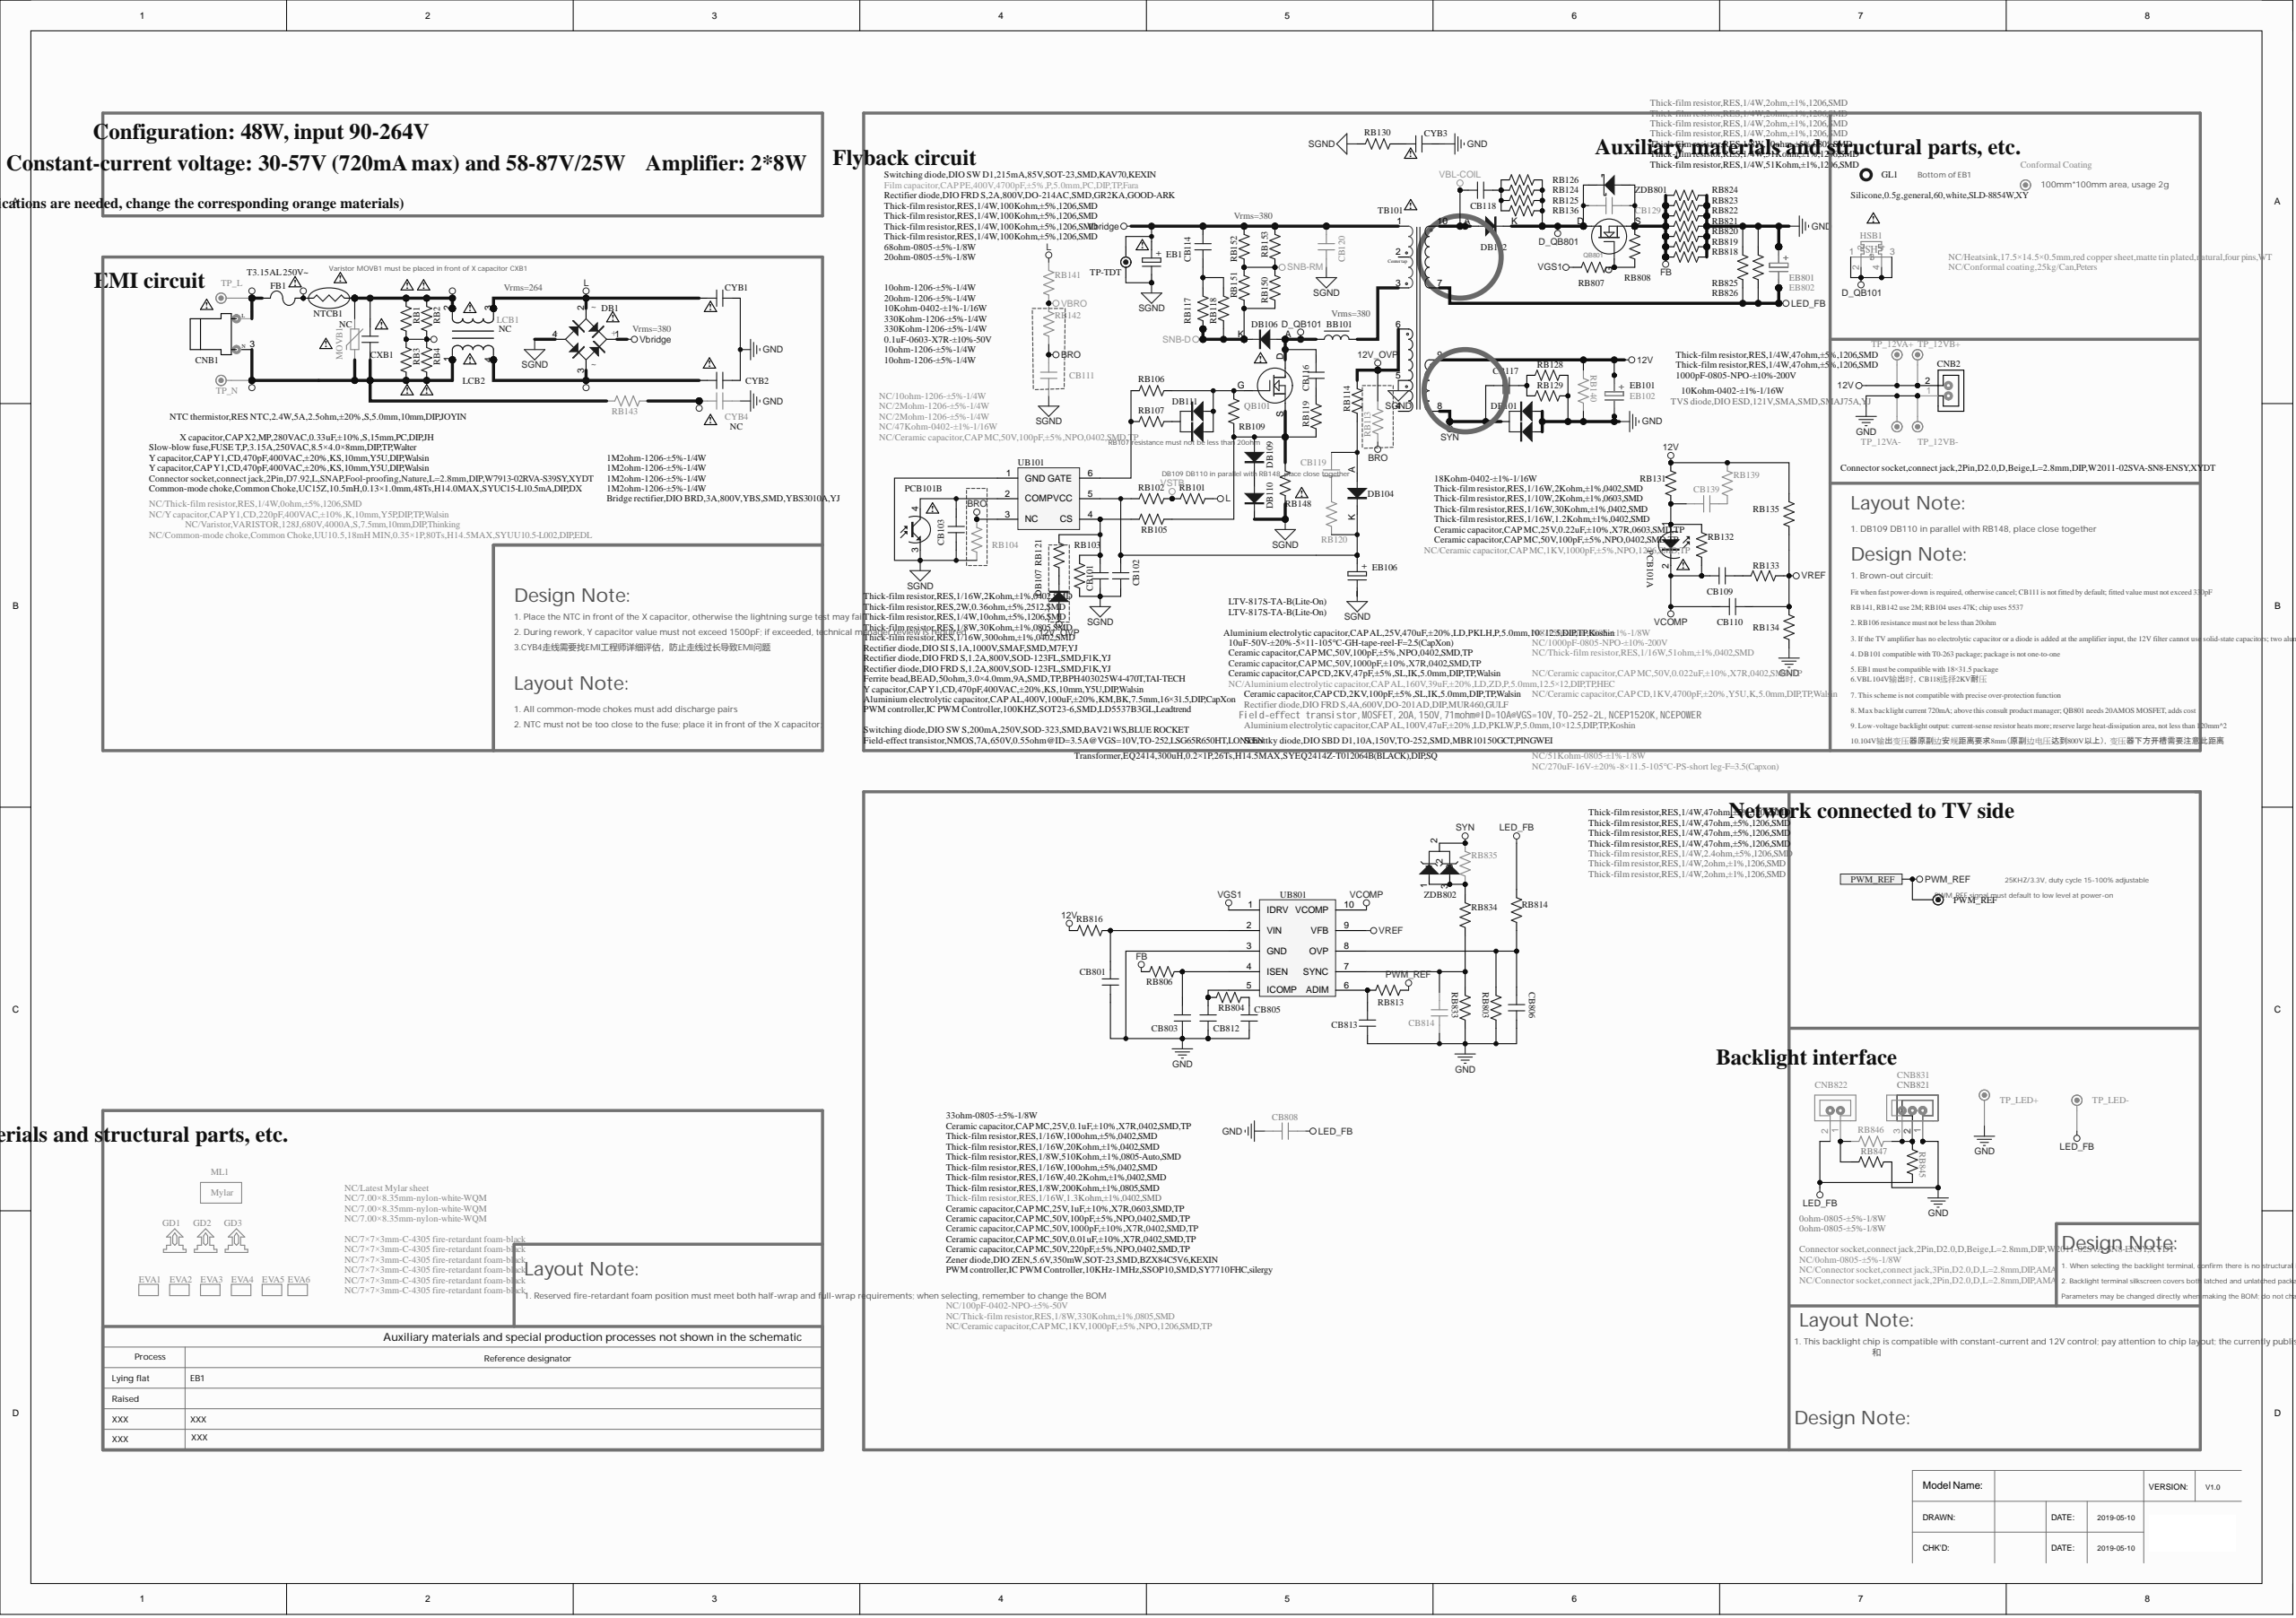Circuit board | Altium Designer | 578 parts | 300 nets | one sheet of the schematic
Parts on this sheet (reference | value | footprint):
BB101 | Ferrite bead,BEAD,50ohm,3.0×4.0mm,9A,SMD,TP,BPH403025W4-470T,TAI-TECH | L(4*3*2.55)-S
CB101 | Ceramic capacitor,CAP MC,50V,100pF,±5%,NPO,0402,SMD,TP | C0402
CB102 | 0.1uF-0603-X7R-±10%-50V | C0603
CB103 | Ceramic capacitor,CAP MC,50V,1000pF,±10%,X7R,0402,SMD,TP | C0402
CB109 | Ceramic capacitor,CAP MC,25V,0.22uF,±10%,X7R,0603,SMD,TP | C0603
CB110 | Ceramic capacitor,CAP MC,50V,100pF,±5%,NPO,0402,SMD,TP | C0402
CB111 | NC/Ceramic capacitor,CAP MC,50V,100pF,±5%,NPO,0402,SMD,TP | C0402
CB114 | Film capacitor,CAP PE,400V,4700pF,±5%,P,5.0mm,PC,DIP,TP,Fara | CAP8*2.5-V-5
CB116 | Ceramic capacitor,CAP CD,2KV,47pF,±5%,SL,IK,5.0mm,DIP,TP,Walsin | CAP7.5*5-V-5-1
CB117 | 1000pF-0805-NPO-±10%-200V | C0805
CB118 | Ceramic capacitor,CAP CD,2KV,100pF,±5%,SL,IK,5.0mm,DIP,TP,Walsin | CAP8.5*5-V-5
CB119 | NC/1000pF-0805-NPO-±10%-200V | C0805
CB120 | NC/Ceramic capacitor,CAP CD,1KV,4700pF,±20%,Y5U,K,5.0mm,DIP,TP,Walsin | CAP10*4.5-V-5
CB129 | NC/Ceramic capacitor,CAP MC,1KV,1000pF,±5%,NPO,1206,SMD,TP | C1206
CB139 | NC/Ceramic capacitor,CAP MC,50V,0.022uF,±10%,X7R,0402,SMD,TP | C0603
CB801 | Ceramic capacitor,CAP MC,25V,1uF,±10%,X7R,0603,SMD,TP | C0603
CB803 | Ceramic capacitor,CAP MC,25V,0.1uF,±10%,X7R,0402,SMD,TP | C0402
CB805 | Ceramic capacitor,CAP MC,50V,0.01uF,±10%,X7R,0402,SMD,TP | C0402
CB806 | Ceramic capacitor,CAP MC,50V,1000pF,±10%,X7R,0402,SMD,TP | C0402
CB808 | NC/Ceramic capacitor,CAP MC,1KV,1000pF,±5%,NPO,1206,SMD,TP | C1206
CB812 | Ceramic capacitor,CAP MC,50V,220pF,±5%,NPO,0402,SMD,TP | C0402
CB813 | Ceramic capacitor,CAP MC,50V,100pF,±5%,NPO,0402,SMD,TP | C0402
CB814 | NC/100pF-0402-NPO-±5%-50V | C0402
CNB1 | Connector socket,connect jack,2Pin,D7.92,L,SNAP,Fool-proofing,Nature,L=2.8mm,DIP,W7913-02RVA-S39SY,XYDT | CON2-H7.92
CNB2 | Connector socket,connect jack,2Pin,D2.0,D,Beige,L=2.8mm,DIP,W2011-02SVA-SN8-ENSY,XYDT | SIP2/2.0D-1
CNB821 | Connector socket,connect jack,2Pin,D2.0,D,Beige,L=2.8mm,DIP,W2011-02SVA-SN8-ENSY,XYDT | SIP2/2.0D-CP
CNB822 | NC/Connector socket,connect jack,2Pin,D2.0,D,L=2.8mm,DIP,AMA | SIP2/2.0D-CP
CNB831 | NC/Connector socket,connect jack,3Pin,D2.0,D,L=2.8mm,DIP,AMA | SIP3/2.0D-CP
CXB1 | X capacitor,CAP X2,MP,280VAC,0.33uF,±10%,S,15mm,PC,DIP,JH | CAP18*8.5-V-15
CYB1 | Y capacitor,CAP Y1,CD,470pF,400VAC,±20%,KS,10mm,Y5U,DIP,Walsin | CAP13*5-V-10-1
CYB2 | Y capacitor,CAP Y1,CD,470pF,400VAC,±20%,KS,10mm,Y5U,DIP,Walsin | CAP13*5-V-10-1
CYB3 | Y capacitor,CAP Y1,CD,470pF,400VAC,±20%,KS,10mm,Y5U,DIP,Walsin | CAP13*5-V-10-1
CYB4 | NC/Y capacitor,CAP Y1,CD,220pF,400VAC,±10%,K,10mm,Y5P,DIP,TP,Walsin | CAP13*5-V-10-1
DB1 | Bridge rectifier,DIO BRD,3A,800V,YBS,SMD,YBS3010A,YJ | B/YBS3010A
DB101 | Schottky diode,DIO SBD D1,10A,150V,TO-252,SMD,MBR10150GCT,PINGWEI | D2PAK3
DB102 | Rectifier diode,DIO FRD S,4A,600V,DO-201AD,DIP,MUR460,GULF | D3-H-20
DB104 | Rectifier diode,DIO SI S,1A,1000V,SMAF,SMD,M7F,YJ | DIODE-S-2
DB106 | Rectifier diode,DIO FRD S,2A,800V,DO-214AC,SMD,GR2KA,GOOD-ARK | DIODE-SMA-2
DB107 | Switching diode,DIO SW S,200mA,250V,SOD-323,SMD,BAV21WS,BLUE ROCKET | DIODE-S-12
DB109 | Rectifier diode,DIO FRD S,1.2A,800V,SOD-123FL,SMD,F1K,YJ | DIODE-S-14
DB110 | Rectifier diode,DIO FRD S,1.2A,800V,SOD-123FL,SMD,F1K,YJ | DIODE-S-14
DB111 | Switching diode,DIO SW D1,215mA,85V,SOT-23,SMD,KAV70,KEXIN | SO-23
EB1 | Aluminium electrolytic capacitor,CAP AL,400V,100uF,±20%,KM,BK,7.5mm,16×31.5,DIP,CapXon | EC(18*31.5)-H-7.5
EB101 | Aluminium electrolytic capacitor,CAP AL,25V,470uF,±20%,LD,PKLH,P,5.0mm,10×12.5,DIP,TP,Koshin | EC(10*12.5)-V-5
EB102 | NC/270uF-16V-±20%-8×11.5-105℃-PS-short leg-F=3.5(Capxon) | EC(8*11)-V-3.5
EB106 | 10uF-50V-±20%-5×11-105℃-GH-tape-reel-F=2.5(CapXon) | EC(5*11)-V-2.5
EB801 | Aluminium electrolytic capacitor,CAP AL,100V,47uF,±20%,LD,PKLW,P,5.0mm,10×12.5,DIP,TP,Koshin | EC(10*12.5)-V-5
EB802 | NC/Aluminium electrolytic capacitor,CAP AL,160V,39uF,±20%,LD,ZD,P,5.0mm,12.5×12,DIP,TP,HEC | EC(13*13)-V-5
EVA1 | NC/7×7×3mm-C-4305 fire-retardant foam-black | EVA(7*7*3)
EVA2 | NC/7×7×3mm-C-4305 fire-retardant foam-black | EVA(7*7*3)
EVA3 | NC/7×7×3mm-C-4305 fire-retardant foam-black | EVA(7*7*3)
EVA4 | NC/7×7×3mm-C-4305 fire-retardant foam-black | EVA(7*7*3)
EVA5 | NC/7×7×3mm-C-4305 fire-retardant foam-black | EVA(7*7*3)
EVA6 | NC/7×7×3mm-C-4305 fire-retardant foam-black | EVA(7*7*3)
FB1 | Slow-blow fuse,FUSE T,P,3.15A,250VAC,8.5×4.0×8mm,DIP,TP,Walter | FUSE8.5*4-V-5(T3.15AL 250V~)
GD1 | NC/7.00×8.35mm-nylon-white-WQM | Fixed
GD2 | NC/7.00×8.35mm-nylon-white-WQM | Fixed
GD3 | NC/7.00×8.35mm-nylon-white-WQM | Fixed
GL1 | Silicone,0.5g,general,60,white,SLD-8854W,XY | Silica gel-15
HSB1 | NC/Heatsink,17.5×14.5×0.5mm,red copper sheet,matte tin plated,natural,four pins,WT | HS149-YZ
LCB1 | NC/Common-mode choke,Common Choke,UU10.5,18mH MIN,0.35×1P,80Ts,H14.5MAX,SYUU10.5-L002,DIP,EDL | L/UU10.5/10*13-2
LCB2 | Common-mode choke,Common Choke,UC15Z,10.5mH,0.13×1.0mm,48Ts,H14.0MAX,SYUC15-L10.5mA,DIP,DX | L/LC4/20.5*16-H-17*9(12.9)
ML1 | NC/Latest Mylar sheet | Mylar
MOVB1 | NC/Varistor,VARISTOR,128J,680V,4000A,S,7.5mm,10mm,DIP,Thinking | VR(13*5)-V-7.5
NTCB1 | NTC thermistor,RES NTC,2.4W,5A,2.5ohm,±20%,S,5.0mm,10mm,DIP,JOYIN | NTC(10*5)-V5
QB101 | Field-effect transistor,NMOS,7A,650V,0.55ohm@ID=3.5A@VGS=10V,TO-252,LSG65R650HT,LONTEN | TO-252-GDS
QB801 | Field-effect transistor,MOSFET,20A,150V,71mohm@ID=10A@VGS=10V,TO-252-2L,NCEP1520K,NCEPOWER | TO-252-GDS
RB1 | 1M2ohm-1206-±5%-1/4W | R1206
RB2 | 1M2ohm-1206-±5%-1/4W | R1206
RB3 | 1M2ohm-1206-±5%-1/4W | R1206
RB4 | 1M2ohm-1206-±5%-1/4W | R1206
RB101 | 330Kohm-1206-±5%-1/4W | R1206
RB102 | 330Kohm-1206-±5%-1/4W | R1206
RB103 | Thick-film resistor,RES,1/16W,2Kohm,±1%,0402,SMD | R0402
RB104 | NC/47Kohm-0402-±1%-1/16W | R0402
RB105 | Thick-film resistor,RES,1/16W,300ohm,±1%,0402,SMD | R0402
RB106 | 68ohm-0805-±5%-1/8W | R0805
RB107 | 20ohm-0805-±5%-1/8W | R0805
RB109 | 10Kohm-0402-±1%-1/16W | R0402
RB113 | NC/150Kohm-0805-±1%-1/8W | R0805
RB114 | Thick-film resistor,RES,1/4W,10ohm,±5%,1206,SMD | R1206
RB117 | 10ohm-1206-±5%-1/4W | R1206
RB118 | 10ohm-1206-±5%-1/4W | R1206
RB119 | 10ohm-1206-±5%-1/4W | R1206
RB120 | NC/10ohm-1206-±5%-1/4W | R1206
RB121 | Thick-film resistor,RES,1/8W,30Kohm,±1%,0805,SMD | R0805
RB124 | Thick-film resistor,RES,1/4W,47ohm,±5%,1206,SMD | R1206
RB125 | Thick-film resistor,RES,1/4W,47ohm,±5%,1206,SMD | R1206
RB126 | Thick-film resistor,RES,1/4W,47ohm,±5%,1206,SMD | R1206
RB128 | Thick-film resistor,RES,1/4W,47ohm,±5%,1206,SMD | R1206
RB129 | Thick-film resistor,RES,1/4W,47ohm,±5%,1206,SMD | R1206
RB130 | 20ohm-1206-±5%-1/4W | R1206
RB131 | Thick-film resistor,RES,1/10W,2Kohm,±1%,0603,SMD | R0603
RB132 | Thick-film resistor,RES,1/16W,1.2Kohm,±1%,0402,SMD | R0402
RB133 | Thick-film resistor,RES,1/16W,30Kohm,±1%,0402,SMD | R0402
RB134 | Thick-film resistor,RES,1/16W,2Kohm,±1%,0402,SMD | R0402
RB135 | 18Kohm-0402-±1%-1/16W | R0402
RB136 | Thick-film resistor,RES,1/4W,47ohm,±5%,1206,SMD | R1206
RB139 | NC/Thick-film resistor,RES,1/16W,51ohm,±1%,0402,SMD | R0402
RB140 | NC/51Kohm-0805-±1%-1/8W | R0805
RB141 | NC/2Mohm-1206-±5%-1/4W | R1206
RB142 | NC/2Mohm-1206-±5%-1/4W | R1206
RB143 | NC/Thick-film resistor,RES,1/4W,0ohm,±5%,1206,SMD | R1206
RB148 | Thick-film resistor,RES,2W,0.36ohm,±5%,2512,SMD | R2512-1
RB150 | Thick-film resistor,RES,1/4W,100Kohm,±5%,1206,SMD | R1206
RB151 | Thick-film resistor,RES,1/4W,100Kohm,±5%,1206,SMD | R1206
RB152 | Thick-film resistor,RES,1/4W,100Kohm,±5%,1206,SMD | R1206
RB153 | Thick-film resistor,RES,1/4W,100Kohm,±5%,1206,SMD | R1206
RB803 | Thick-film resistor,RES,1/16W,1.3Kohm,±1%,0402,SMD | R0402
RB804 | Thick-film resistor,RES,1/16W,20Kohm,±1%,0402,SMD | R0402
RB806 | Thick-film resistor,RES,1/16W,100ohm,±5%,0402,SMD | R0402
RB807 | Thick-film resistor,RES,1/8W,10ohm,±5%,0805,SMD | R0805
RB808 | 10Kohm-0402-±1%-1/16W | R0402
RB813 | Thick-film resistor,RES,1/16W,100ohm,±5%,0402,SMD | R0402
RB814 | Thick-film resistor,RES,1/8W,510Kohm,±1%,0805-Auto,SMD | R0805
RB816 | 33ohm-0805-±5%-1/8W | R0805
RB818 | Thick-film resistor,RES,1/4W,2ohm,±1%,1206,SMD | R1206
RB819 | Thick-film resistor,RES,1/4W,2ohm,±1%,1206,SMD | R1206
RB820 | Thick-film resistor,RES,1/4W,2ohm,±1%,1206,SMD | R1206
RB821 | Thick-film resistor,RES,1/4W,2ohm,±1%,1206,SMD | R1206
RB822 | Thick-film resistor,RES,1/4W,2ohm,±1%,1206,SMD | R1206
RB823 | Thick-film resistor,RES,1/4W,2ohm,±1%,1206,SMD | R1206
RB824 | Thick-film resistor,RES,1/4W,2.4ohm,±5%,1206,SMD | R1206
RB825 | Thick-film resistor,RES,1/4W,51Kohm,±1%,1206,SMD | R1206
RB826 | Thick-film resistor,RES,1/4W,51Kohm,±1%,1206,SMD | R1206
RB833 | Thick-film resistor,RES,1/16W,40.2Kohm,±1%,0402,SMD | R0402
RB834 | Thick-film resistor,RES,1/8W,200Kohm,±1%,0805,SMD | R0805
RB835 | NC/Thick-film resistor,RES,1/8W,330Kohm,±1%,0805,SMD | R0805
RB845 | 0ohm-0805-±5%-1/8W | R0805
RB846 | NC/0ohm-0805-±5%-1/8W | R0805
RB847 | 0ohm-0805-±5%-1/8W | R0805
TB101 | Transformer,EQ2414,300uH,0.2×1P,26Ts,H14.5MAX,SYEQ2414Z-T012064B(BLACK),DIP,SQ | T/EQ2414*10
TP-TDT | TP-TDT
TP_12VA+ | NC/ | TP
TP_12VA- | NC/ | TP
TP_L | NC/ | TP-80
TP_LED+ | NC/ | TP
TP_N | NC/ | TP-80
UB101 | PWM controller,IC PWM Controller,100KHZ,SOT23-6,SMD,LD5537B3GL,Leadtrend | SOT-26
UB801 | PWM controller,IC PWM Controller,10KHz-1MHz,SSOP10,SMD,SY7710FHC,silergy | SOP10/1.0-1
ZDB801 | TVS diode,DIO ESD,121V,SMA,SMD,SMAJ75A,YJ | DIODE-SMA-1
ZDB802 | Zener diode,DIO ZEN,5.6V,350mW,SOT-23,SMD,BZX84C5V6,KEXIN | SO-23
Nets of these parts (net: part-pin ...):
VSTB: RB101-2 RB102-2
VREF: CB110-2 RB133-1 RB134-2 RB135-2 UB801-9
VGS1: RB807-1 UB801-1
VCOMP: CB109-1 CB110-1 RB132-1 UB801-10
VBRO: RB141-1 RB142-2
Vbridge: CB114-1 CB120-2 DB1-1 EB1-1 RB152-2 RB153-2 TB101-1 TP-TDT-1
VBL-COIL: CB118-1 DB102-A TB101-10
SYN: CB117-1 DB101-2 RB835-1 TB101-8 ZDB802-2
SNB-RM: RB150-2 RB151-2 RB152-1 RB153-1
SNB-D: DB106-K RB117-1 RB118-1 RB150-1 RB151-1
SGND: CB101-2 CB102-2 CB103-2 CB111-1 CB120-1 DB1-4 DB110-K EB1-2 EB106-2 RB103-1 RB104-1 RB130-1 RB148-1 TB101-5 TP-TDT-2 UB101-1
PWM_REF: RB813-1
NetRB834_2: RB834-2 RB835-2 ZDB802-1 ZDB802-3
NetRB106_1: RB106-1 RB107-1 UB101-6
NetQB801_G: QB801-G RB807-2 RB808-1
NetDB111_2: DB111-2 RB107-2
NetDB111_1: DB111-1 DB111-3 QB101-G RB106-2 RB109-2
NetDB109_K: DB109-K DB110-A
NetDB109_A: DB109-A QB101-S RB105-2 RB109-1 RB119-1 RB148-2
NetDB107_K: DB107-K RB121-1
NetCYB3_1: CYB3-1 RB130-2
NetCNB822_1: CNB822-1 RB846-2 RB847-2
NetCNB821_2: CNB821-2 CNB831-2 CNB831-3 RB845-2 RB846-1
NetCB814_1: CB814-1 RB833-2 RB834-1 UB801-7
NetCB813_2: CB813-2 RB813-2 UB801-6
NetCB812_2: CB812-2 RB804-2 UB801-5
NetCB806_1: CB806-1 RB803-2 RB814-2 UB801-8
NetCB805_2: CB805-2 RB804-1
NetCB803_1: CB803-1 RB806-2 UB801-4
NetCB801_1: CB801-1 RB816-2 UB801-2
NetCB139_2: CB139-2 RB131-1 RB132-2
NetCB139_1: CB139-1 RB139-2
NetCB119_2: CB119-2 DB104-A RB114-1
NetCB119_1: CB119-1 RB120-2
NetCB118_2: CB118-2 RB124-2 RB125-2 RB126-2 RB136-2
NetCB117_2: CB117-2 RB128-1 RB129-1
NetCB116_2: CB116-2 RB119-2
NetCB114_2: CB114-2 RB117-2 RB118-2
NetCB109_2: CB109-2 RB133-2
NetCB103_1: CB103-1 UB101-2
NetCB102_1: CB102-1 DB104-K EB106-1 RB102-1 RB120-1 UB101-5
NetCB101_1: CB101-1 RB103-2 RB105-1 RB121-2 UB101-4
NetBB101_2: BB101-2 TB101-3
N-3: CYB4-1 RB143-2
N-2: CYB2-1 DB1-3 LCB1-4 LCB2-4
N-1: CNB1-3 CXB1-2 LCB1-1 LCB2-1 MOVB1-2 RB3-2 RB4-2 RB143-1 TP_N-1
LED_FB: CB808-2 CNB822-2 EB801-2 EB802-2 RB814-1 RB825-2 RB826-2 RB845-1 TB101-7
L-N: RB1-2 RB2-2 RB3-1 RB4-1
L-3: CXB1-1 LCB1-2 LCB2-2 MOVB1-1 NTCB1-2 RB1-1 RB2-1
L-2: FB1-2 NTCB1-1
L-1: CNB1-1 FB1-1 TP_L-1
L: CYB1-1 DB1-2 LCB1-3 LCB2-3 RB101-1 RB141-2
GND: CB801-2 CB803-2 CB805-1 CB806-2 CB808-1 CB812-1 CB813-1 CB814-2 CNB2-1 CNB821-1 CNB831-1 CYB1-2 CYB2-2 CYB3-2 CYB4-2 DB101-1 DB101-3 EB101-2 EB102-2 EB801-1 EB802-1 RB128-2 RB129-2 RB134-1 RB140-2 RB803-1 RB818-2 RB819-2 RB820-2 RB821-2 RB822-2 RB823-2 RB824-2 RB825-1 RB826-1 RB833-1 RB847-1 TP_12VA--1 TP_LED+-1 UB801-3
FB: CB129-2 QB801-S RB806-1 RB808-2 RB818-1 RB819-1 RB820-1 RB821-1 RB822-1 RB823-1 RB824-1 ZDB801-A
D_QB801: CB129-1 DB102-K QB801-D RB124-1 RB125-1 RB126-1 RB136-1 ZDB801-K
D_QB101: BB101-1 CB116-1 DB106-A HSB1-1 HSB1-2 HSB1-3 HSB1-4 QB101-D
BRO: CB111-2 RB104-2 RB113-1 RB142-1 UB101-3
12V_OVP: DB107-A RB113-2 RB114-2 TB101-6
12V: CNB2-2 EB101-1 EB102-1 RB131-2 RB135-1 RB139-1 RB140-1 RB816-1 TB101-9 TP_12VA+-1